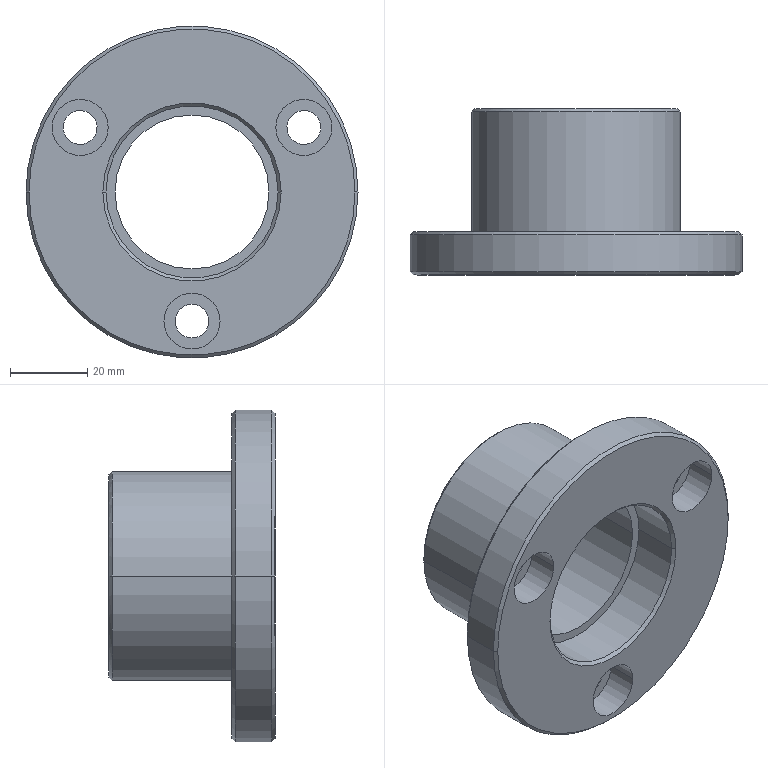Part | Creo | features CUT 4, CURVE 3, DATUM PLANE 3, CHAMFER 1, COORDINATE SYSTEM 1, PATTERN 1, PROTRUSION 1 | 1 solid | 40 faces | box 85.764 x 42.882 x 85.764 mm | volume 70979 mm3 | cylinder 22 | cone 10 | plane 8 | commonest cylinder face diameters 8.735 x6 14.5 x6 44.47 x4 39.777 x2 54 x2 85.764 x2
STEP:
#1=CARTESIAN_POINT('',(0.,0.,0.));
#2=DIRECTION('',(0.,0.,1.));
#3=DIRECTION('',(1.,0.,0.));
#4=AXIS2_PLACEMENT_3D('',#1,#2,#3);
#5=CARTESIAN_POINT('',(22.235,0.7941,0.));
#6=VERTEX_POINT('',#5);
#7=CARTESIAN_POINT('',(-22.235,0.7941,0.));
#8=VERTEX_POINT('',#7);
#9=CARTESIAN_POINT('',(0.,0.7941,0.));
#10=DIRECTION('',(0.,1.,0.));
#11=DIRECTION('',(1.,0.,0.));
#12=AXIS2_PLACEMENT_3D('',#9,#10,#11);
#13=CIRCLE('',#12,22.235);
#14=EDGE_CURVE('',#6,#8,#13,.T.);
#15=ORIENTED_EDGE('',*,*,#14,.T.);
#16=CARTESIAN_POINT('',(-22.235,12.706,0.));
#17=VERTEX_POINT('',#16);
#18=CARTESIAN_POINT('',(-22.235,12.706,0.));
#19=DIRECTION('',(0.,-1.,0.000000001));
#20=VECTOR('',#19,11.912);
#21=LINE('',#18,#20);
#22=EDGE_CURVE('',#17,#8,#21,.T.);
#23=ORIENTED_EDGE('',*,*,#22,.F.);
#24=CARTESIAN_POINT('',(22.235,12.706,0.));
#25=VERTEX_POINT('',#24);
#26=CARTESIAN_POINT('',(0.,12.706,0.));
#27=DIRECTION('',(0.,1.,0.));
#28=DIRECTION('',(1.,0.,0.));
#29=AXIS2_PLACEMENT_3D('',#26,#27,#28);
#30=CIRCLE('',#29,22.235);
#31=EDGE_CURVE('',#25,#17,#30,.T.);
#32=ORIENTED_EDGE('',*,*,#31,.F.);
#33=CARTESIAN_POINT('',(22.235,12.706,0.));
#34=DIRECTION('',(0.,-1.,-0.000000001));
#35=VECTOR('',#34,11.912);
#36=LINE('',#33,#35);
#37=EDGE_CURVE('',#25,#6,#36,.T.);
#38=ORIENTED_EDGE('',*,*,#37,.T.);
#39=EDGE_LOOP('',(#15,#23,#32,#38));
#40=FACE_OUTER_BOUND('',#39,.F.);
#41=CARTESIAN_POINT('',(0.,0.,0.));
#42=DIRECTION('',(0.,1.,0.));
#43=DIRECTION('',(1.,0.,0.));
#44=AXIS2_PLACEMENT_3D('',#41,#42,#43);
#45=CYLINDRICAL_SURFACE('',#44,22.235);
#46=ADVANCED_FACE('',(#40),#45,.F.);
#47=CARTESIAN_POINT('',(23.029,0.,0.));
#48=VERTEX_POINT('',#47);
#49=CARTESIAN_POINT('',(-23.029,0.,0.));
#50=VERTEX_POINT('',#49);
#51=CARTESIAN_POINT('',(0.,0.,0.));
#52=DIRECTION('',(0.,1.,0.));
#53=DIRECTION('',(1.,0.,0.));
#54=AXIS2_PLACEMENT_3D('',#51,#52,#53);
#55=CIRCLE('',#54,23.029);
#56=EDGE_CURVE('',#48,#50,#55,.T.);
#57=ORIENTED_EDGE('',*,*,#56,.T.);
#58=CARTESIAN_POINT('',(-23.029,0.000000001,0.000000013));
#59=DIRECTION('',(0.7071,0.7071,-0.000000003));
#60=VECTOR('',#59,1.123);
#61=LINE('',#58,#60);
#62=EDGE_CURVE('',#50,#8,#61,.T.);
#63=ORIENTED_EDGE('',*,*,#62,.T.);
#64=ORIENTED_EDGE('',*,*,#14,.F.);
#65=CARTESIAN_POINT('',(23.029,0.000000001,-0.000000013));
#66=DIRECTION('',(-0.7071,0.7071,0.000000003));
#67=VECTOR('',#66,1.123);
#68=LINE('',#65,#67);
#69=EDGE_CURVE('',#48,#6,#68,.T.);
#70=ORIENTED_EDGE('',*,*,#69,.F.);
#71=EDGE_LOOP('',(#57,#63,#64,#70));
#72=FACE_OUTER_BOUND('',#71,.F.);
#73=CARTESIAN_POINT('',(0.,0.3971,0.));
#74=DIRECTION('',(0.,-1.,0.));
#75=DIRECTION('',(0.,0.,-1.));
#76=AXIS2_PLACEMENT_3D('',#73,#74,#75);
#77=CONICAL_SURFACE('',#76,22.632,45.);
#78=ADVANCED_FACE('',(#72),#77,.F.);
#79=CARTESIAN_POINT('',(-42.088,0.,0.));
#80=VERTEX_POINT('',#79);
#81=CARTESIAN_POINT('',(42.088,0.,0.));
#82=VERTEX_POINT('',#81);
#83=CARTESIAN_POINT('',(0.,0.,0.));
#84=DIRECTION('',(0.,1.,0.));
#85=DIRECTION('',(-1.,0.,0.));
#86=AXIS2_PLACEMENT_3D('',#83,#84,#85);
#87=CIRCLE('',#86,42.088);
#88=EDGE_CURVE('',#80,#82,#87,.T.);
#89=ORIENTED_EDGE('',*,*,#88,.T.);
#90=CARTESIAN_POINT('',(0.,0.,0.));
#91=DIRECTION('',(0.,1.,0.));
#92=DIRECTION('',(1.,0.,0.));
#93=AXIS2_PLACEMENT_3D('',#90,#91,#92);
#94=CIRCLE('',#93,42.088);
#95=EDGE_CURVE('',#82,#80,#94,.T.);
#96=ORIENTED_EDGE('',*,*,#95,.T.);
#97=EDGE_LOOP('',(#89,#96));
#98=FACE_OUTER_BOUND('',#97,.F.);
#99=CARTESIAN_POINT('',(21.634,0.,16.676));
#100=VERTEX_POINT('',#99);
#101=CARTESIAN_POINT('',(36.134,0.,16.676));
#102=VERTEX_POINT('',#101);
#103=CARTESIAN_POINT('',(28.884,0.,16.676));
#104=DIRECTION('',(0.,-1.,0.));
#105=DIRECTION('',(-1.,0.,0.));
#106=AXIS2_PLACEMENT_3D('',#103,#104,#105);
#107=CIRCLE('',#106,7.25);
#108=EDGE_CURVE('',#100,#102,#107,.T.);
#109=ORIENTED_EDGE('',*,*,#108,.T.);
#110=CARTESIAN_POINT('',(28.884,0.,16.676));
#111=DIRECTION('',(0.,-1.,0.));
#112=DIRECTION('',(1.,0.,0.));
#113=AXIS2_PLACEMENT_3D('',#110,#111,#112);
#114=CIRCLE('',#113,7.25);
#115=EDGE_CURVE('',#102,#100,#114,.T.);
#116=ORIENTED_EDGE('',*,*,#115,.T.);
#117=EDGE_LOOP('',(#109,#116));
#118=FACE_BOUND('',#117,.F.);
#119=CARTESIAN_POINT('',(-36.134,0.,16.676));
#120=VERTEX_POINT('',#119);
#121=CARTESIAN_POINT('',(-21.634,0.,16.676));
#122=VERTEX_POINT('',#121);
#123=CARTESIAN_POINT('',(-28.884,0.,16.676));
#124=DIRECTION('',(0.,-1.,0.));
#125=DIRECTION('',(-1.,0.,0.));
#126=AXIS2_PLACEMENT_3D('',#123,#124,#125);
#127=CIRCLE('',#126,7.25);
#128=EDGE_CURVE('',#120,#122,#127,.T.);
#129=ORIENTED_EDGE('',*,*,#128,.T.);
#130=CARTESIAN_POINT('',(-28.884,0.,16.676));
#131=DIRECTION('',(0.,-1.,0.));
#132=DIRECTION('',(1.,0.,0.));
#133=AXIS2_PLACEMENT_3D('',#130,#131,#132);
#134=CIRCLE('',#133,7.25);
#135=EDGE_CURVE('',#122,#120,#134,.T.);
#136=ORIENTED_EDGE('',*,*,#135,.T.);
#137=EDGE_LOOP('',(#129,#136));
#138=FACE_BOUND('',#137,.F.);
#139=CARTESIAN_POINT('',(-7.25,0.,-33.353));
#140=VERTEX_POINT('',#139);
#141=CARTESIAN_POINT('',(7.25,0.,-33.353));
#142=VERTEX_POINT('',#141);
#143=CARTESIAN_POINT('',(0.,0.,-33.353));
#144=DIRECTION('',(0.,-1.,0.));
#145=DIRECTION('',(-1.,0.,0.));
#146=AXIS2_PLACEMENT_3D('',#143,#144,#145);
#147=CIRCLE('',#146,7.25);
#148=EDGE_CURVE('',#140,#142,#147,.T.);
#149=ORIENTED_EDGE('',*,*,#148,.T.);
#150=CARTESIAN_POINT('',(0.,0.,-33.353));
#151=DIRECTION('',(0.,-1.,0.));
#152=DIRECTION('',(1.,0.,0.));
#153=AXIS2_PLACEMENT_3D('',#150,#151,#152);
#154=CIRCLE('',#153,7.25);
#155=EDGE_CURVE('',#142,#140,#154,.T.);
#156=ORIENTED_EDGE('',*,*,#155,.T.);
#157=EDGE_LOOP('',(#149,#156));
#158=FACE_BOUND('',#157,.F.);
#159=CARTESIAN_POINT('',(0.,0.,0.));
#160=DIRECTION('',(0.,1.,0.));
#161=DIRECTION('',(-1.,0.,0.));
#162=AXIS2_PLACEMENT_3D('',#159,#160,#161);
#163=CIRCLE('',#162,23.029);
#164=EDGE_CURVE('',#50,#48,#163,.T.);
#165=ORIENTED_EDGE('',*,*,#164,.F.);
#166=ORIENTED_EDGE('',*,*,#56,.F.);
#167=EDGE_LOOP('',(#165,#166));
#168=FACE_BOUND('',#167,.F.);
#169=CARTESIAN_POINT('',(0.,0.,0.));
#170=DIRECTION('',(0.,1.,0.));
#171=DIRECTION('',(1.,0.,0.));
#172=AXIS2_PLACEMENT_3D('',#169,#170,#171);
#173=PLANE('',#172);
#174=ADVANCED_FACE('',(#98,#118,#138,#158,#168),#173,.F.);
#175=ORIENTED_EDGE('',*,*,#148,.F.);
#176=CARTESIAN_POINT('',(-7.25,7.941,-33.353));
#177=VERTEX_POINT('',#176);
#178=CARTESIAN_POINT('',(-7.25,0.,-33.353));
#179=DIRECTION('',(0.,1.,0.));
#180=VECTOR('',#179,7.941);
#181=LINE('',#178,#180);
#182=EDGE_CURVE('',#140,#177,#181,.T.);
#183=ORIENTED_EDGE('',*,*,#182,.T.);
#184=CARTESIAN_POINT('',(7.25,7.941,-33.353));
#185=VERTEX_POINT('',#184);
#186=CARTESIAN_POINT('',(0.,7.941,-33.353));
#187=DIRECTION('',(0.,-1.,0.));
#188=DIRECTION('',(-1.,0.,0.));
#189=AXIS2_PLACEMENT_3D('',#186,#187,#188);
#190=CIRCLE('',#189,7.25);
#191=EDGE_CURVE('',#177,#185,#190,.T.);
#192=ORIENTED_EDGE('',*,*,#191,.T.);
#193=CARTESIAN_POINT('',(7.25,0.,-33.353));
#194=DIRECTION('',(0.,1.,0.));
#195=VECTOR('',#194,7.941);
#196=LINE('',#193,#195);
#197=EDGE_CURVE('',#142,#185,#196,.T.);
#198=ORIENTED_EDGE('',*,*,#197,.F.);
#199=EDGE_LOOP('',(#175,#183,#192,#198));
#200=FACE_OUTER_BOUND('',#199,.F.);
#201=CARTESIAN_POINT('',(0.,0.,-33.353));
#202=DIRECTION('',(0.,-1.,0.));
#203=DIRECTION('',(-1.,0.,0.));
#204=AXIS2_PLACEMENT_3D('',#201,#202,#203);
#205=CYLINDRICAL_SURFACE('',#204,7.25);
#206=ADVANCED_FACE('',(#200),#205,.F.);
#207=ORIENTED_EDGE('',*,*,#155,.F.);
#208=ORIENTED_EDGE('',*,*,#197,.T.);
#209=CARTESIAN_POINT('',(0.,7.941,-33.353));
#210=DIRECTION('',(0.,-1.,0.));
#211=DIRECTION('',(1.,0.,0.));
#212=AXIS2_PLACEMENT_3D('',#209,#210,#211);
#213=CIRCLE('',#212,7.25);
#214=EDGE_CURVE('',#185,#177,#213,.T.);
#215=ORIENTED_EDGE('',*,*,#214,.T.);
#216=ORIENTED_EDGE('',*,*,#182,.F.);
#217=EDGE_LOOP('',(#207,#208,#215,#216));
#218=FACE_OUTER_BOUND('',#217,.F.);
#219=CARTESIAN_POINT('',(0.,0.,-33.353));
#220=DIRECTION('',(0.,-1.,0.));
#221=DIRECTION('',(-1.,0.,0.));
#222=AXIS2_PLACEMENT_3D('',#219,#220,#221);
#223=CYLINDRICAL_SURFACE('',#222,7.25);
#224=ADVANCED_FACE('',(#218),#223,.F.);
#225=ORIENTED_EDGE('',*,*,#191,.F.);
#226=ORIENTED_EDGE('',*,*,#214,.F.);
#227=EDGE_LOOP('',(#225,#226));
#228=FACE_OUTER_BOUND('',#227,.F.);
#229=CARTESIAN_POINT('',(4.368,7.941,-33.353));
#230=VERTEX_POINT('',#229);
#231=CARTESIAN_POINT('',(-4.368,7.941,-33.353));
#232=VERTEX_POINT('',#231);
#233=CARTESIAN_POINT('',(0.,7.941,-33.353));
#234=DIRECTION('',(0.,1.,0.));
#235=DIRECTION('',(1.,0.,0.));
#236=AXIS2_PLACEMENT_3D('',#233,#234,#235);
#237=CIRCLE('',#236,4.368);
#238=EDGE_CURVE('',#230,#232,#237,.T.);
#239=ORIENTED_EDGE('',*,*,#238,.F.);
#240=CARTESIAN_POINT('',(0.,7.941,-33.353));
#241=DIRECTION('',(0.,1.,0.));
#242=DIRECTION('',(-1.,0.,0.));
#243=AXIS2_PLACEMENT_3D('',#240,#241,#242);
#244=CIRCLE('',#243,4.368);
#245=EDGE_CURVE('',#232,#230,#244,.T.);
#246=ORIENTED_EDGE('',*,*,#245,.F.);
#247=EDGE_LOOP('',(#239,#246));
#248=FACE_BOUND('',#247,.F.);
#249=CARTESIAN_POINT('',(0.,7.941,0.));
#250=DIRECTION('',(0.,-1.,0.));
#251=DIRECTION('',(-1.,0.,0.));
#252=AXIS2_PLACEMENT_3D('',#249,#250,#251);
#253=PLANE('',#252);
#254=ADVANCED_FACE('',(#228,#248),#253,.T.);
#255=CARTESIAN_POINT('',(21.634,7.941,16.676));
#256=VERTEX_POINT('',#255);
#257=CARTESIAN_POINT('',(36.134,7.941,16.676));
#258=VERTEX_POINT('',#257);
#259=CARTESIAN_POINT('',(28.884,7.941,16.676));
#260=DIRECTION('',(0.,-1.,0.));
#261=DIRECTION('',(-1.,0.,0.));
#262=AXIS2_PLACEMENT_3D('',#259,#260,#261);
#263=CIRCLE('',#262,7.25);
#264=EDGE_CURVE('',#256,#258,#263,.T.);
#265=ORIENTED_EDGE('',*,*,#264,.F.);
#266=CARTESIAN_POINT('',(28.884,7.941,16.676));
#267=DIRECTION('',(0.,-1.,0.));
#268=DIRECTION('',(1.,0.,0.));
#269=AXIS2_PLACEMENT_3D('',#266,#267,#268);
#270=CIRCLE('',#269,7.25);
#271=EDGE_CURVE('',#258,#256,#270,.T.);
#272=ORIENTED_EDGE('',*,*,#271,.F.);
#273=EDGE_LOOP('',(#265,#272));
#274=FACE_OUTER_BOUND('',#273,.F.);
#275=CARTESIAN_POINT('',(26.701,7.941,20.459));
#276=VERTEX_POINT('',#275);
#277=CARTESIAN_POINT('',(31.068,7.941,12.894));
#278=VERTEX_POINT('',#277);
#279=CARTESIAN_POINT('',(28.884,7.941,16.676));
#280=DIRECTION('',(0.,1.,0.));
#281=DIRECTION('',(-0.5,0.,0.866));
#282=AXIS2_PLACEMENT_3D('',#279,#280,#281);
#283=CIRCLE('',#282,4.368);
#284=EDGE_CURVE('',#276,#278,#283,.T.);
#285=ORIENTED_EDGE('',*,*,#284,.F.);
#286=CARTESIAN_POINT('',(28.884,7.941,16.676));
#287=DIRECTION('',(0.,1.,0.));
#288=DIRECTION('',(0.5,0.,-0.866));
#289=AXIS2_PLACEMENT_3D('',#286,#287,#288);
#290=CIRCLE('',#289,4.368);
#291=EDGE_CURVE('',#278,#276,#290,.T.);
#292=ORIENTED_EDGE('',*,*,#291,.F.);
#293=EDGE_LOOP('',(#285,#292));
#294=FACE_BOUND('',#293,.F.);
#295=CARTESIAN_POINT('',(0.,7.941,0.));
#296=DIRECTION('',(0.,-1.,0.));
#297=DIRECTION('',(-1.,0.,0.));
#298=AXIS2_PLACEMENT_3D('',#295,#296,#297);
#299=PLANE('',#298);
#300=ADVANCED_FACE('',(#274,#294),#299,.T.);
#301=CARTESIAN_POINT('',(-36.134,7.941,16.676));
#302=VERTEX_POINT('',#301);
#303=CARTESIAN_POINT('',(-21.634,7.941,16.676));
#304=VERTEX_POINT('',#303);
#305=CARTESIAN_POINT('',(-28.884,7.941,16.676));
#306=DIRECTION('',(0.,-1.,0.));
#307=DIRECTION('',(-1.,0.,0.));
#308=AXIS2_PLACEMENT_3D('',#305,#306,#307);
#309=CIRCLE('',#308,7.25);
#310=EDGE_CURVE('',#302,#304,#309,.T.);
#311=ORIENTED_EDGE('',*,*,#310,.F.);
#312=CARTESIAN_POINT('',(-28.884,7.941,16.676));
#313=DIRECTION('',(0.,-1.,0.));
#314=DIRECTION('',(1.,0.,0.));
#315=AXIS2_PLACEMENT_3D('',#312,#313,#314);
#316=CIRCLE('',#315,7.25);
#317=EDGE_CURVE('',#304,#302,#316,.T.);
#318=ORIENTED_EDGE('',*,*,#317,.F.);
#319=EDGE_LOOP('',(#311,#318));
#320=FACE_OUTER_BOUND('',#319,.F.);
#321=CARTESIAN_POINT('',(-31.068,7.941,12.894));
#322=VERTEX_POINT('',#321);
#323=CARTESIAN_POINT('',(-26.701,7.941,20.459));
#324=VERTEX_POINT('',#323);
#325=CARTESIAN_POINT('',(-28.884,7.941,16.676));
#326=DIRECTION('',(0.,1.,0.));
#327=DIRECTION('',(-0.5,0.,-0.866));
#328=AXIS2_PLACEMENT_3D('',#325,#326,#327);
#329=CIRCLE('',#328,4.368);
#330=EDGE_CURVE('',#322,#324,#329,.T.);
#331=ORIENTED_EDGE('',*,*,#330,.F.);
#332=CARTESIAN_POINT('',(-28.884,7.941,16.676));
#333=DIRECTION('',(0.,1.,0.));
#334=DIRECTION('',(0.5,0.,0.866));
#335=AXIS2_PLACEMENT_3D('',#332,#333,#334);
#336=CIRCLE('',#335,4.368);
#337=EDGE_CURVE('',#324,#322,#336,.T.);
#338=ORIENTED_EDGE('',*,*,#337,.F.);
#339=EDGE_LOOP('',(#331,#338));
#340=FACE_BOUND('',#339,.F.);
#341=CARTESIAN_POINT('',(0.,7.941,0.));
#342=DIRECTION('',(0.,-1.,0.));
#343=DIRECTION('',(-1.,0.,0.));
#344=AXIS2_PLACEMENT_3D('',#341,#342,#343);
#345=PLANE('',#344);
#346=ADVANCED_FACE('',(#320,#340),#345,.T.);
#347=ORIENTED_EDGE('',*,*,#108,.F.);
#348=CARTESIAN_POINT('',(21.634,0.,16.676));
#349=DIRECTION('',(0.,1.,0.));
#350=VECTOR('',#349,7.941);
#351=LINE('',#348,#350);
#352=EDGE_CURVE('',#100,#256,#351,.T.);
#353=ORIENTED_EDGE('',*,*,#352,.T.);
#354=ORIENTED_EDGE('',*,*,#264,.T.);
#355=CARTESIAN_POINT('',(36.134,0.,16.676));
#356=DIRECTION('',(0.,1.,0.));
#357=VECTOR('',#356,7.941);
#358=LINE('',#355,#357);
#359=EDGE_CURVE('',#102,#258,#358,.T.);
#360=ORIENTED_EDGE('',*,*,#359,.F.);
#361=EDGE_LOOP('',(#347,#353,#354,#360));
#362=FACE_OUTER_BOUND('',#361,.F.);
#363=CARTESIAN_POINT('',(28.884,0.,16.676));
#364=DIRECTION('',(0.,-1.,0.));
#365=DIRECTION('',(-1.,0.,0.));
#366=AXIS2_PLACEMENT_3D('',#363,#364,#365);
#367=CYLINDRICAL_SURFACE('',#366,7.25);
#368=ADVANCED_FACE('',(#362),#367,.F.);
#369=ORIENTED_EDGE('',*,*,#115,.F.);
#370=ORIENTED_EDGE('',*,*,#359,.T.);
#371=ORIENTED_EDGE('',*,*,#271,.T.);
#372=ORIENTED_EDGE('',*,*,#352,.F.);
#373=EDGE_LOOP('',(#369,#370,#371,#372));
#374=FACE_OUTER_BOUND('',#373,.F.);
#375=CARTESIAN_POINT('',(28.884,0.,16.676));
#376=DIRECTION('',(0.,-1.,0.));
#377=DIRECTION('',(-1.,0.,0.));
#378=AXIS2_PLACEMENT_3D('',#375,#376,#377);
#379=CYLINDRICAL_SURFACE('',#378,7.25);
#380=ADVANCED_FACE('',(#374),#379,.F.);
#381=ORIENTED_EDGE('',*,*,#128,.F.);
#382=CARTESIAN_POINT('',(-36.134,0.,16.676));
#383=DIRECTION('',(0.,1.,0.));
#384=VECTOR('',#383,7.941);
#385=LINE('',#382,#384);
#386=EDGE_CURVE('',#120,#302,#385,.T.);
#387=ORIENTED_EDGE('',*,*,#386,.T.);
#388=ORIENTED_EDGE('',*,*,#310,.T.);
#389=CARTESIAN_POINT('',(-21.634,0.,16.676));
#390=DIRECTION('',(0.,1.,0.));
#391=VECTOR('',#390,7.941);
#392=LINE('',#389,#391);
#393=EDGE_CURVE('',#122,#304,#392,.T.);
#394=ORIENTED_EDGE('',*,*,#393,.F.);
#395=EDGE_LOOP('',(#381,#387,#388,#394));
#396=FACE_OUTER_BOUND('',#395,.F.);
#397=CARTESIAN_POINT('',(-28.884,0.,16.676));
#398=DIRECTION('',(0.,-1.,0.));
#399=DIRECTION('',(-1.,0.,0.));
#400=AXIS2_PLACEMENT_3D('',#397,#398,#399);
#401=CYLINDRICAL_SURFACE('',#400,7.25);
#402=ADVANCED_FACE('',(#396),#401,.F.);
#403=ORIENTED_EDGE('',*,*,#135,.F.);
#404=ORIENTED_EDGE('',*,*,#393,.T.);
#405=ORIENTED_EDGE('',*,*,#317,.T.);
#406=ORIENTED_EDGE('',*,*,#386,.F.);
#407=EDGE_LOOP('',(#403,#404,#405,#406));
#408=FACE_OUTER_BOUND('',#407,.F.);
#409=CARTESIAN_POINT('',(-28.884,0.,16.676));
#410=DIRECTION('',(0.,-1.,0.));
#411=DIRECTION('',(-1.,0.,0.));
#412=AXIS2_PLACEMENT_3D('',#409,#410,#411);
#413=CYLINDRICAL_SURFACE('',#412,7.25);
#414=ADVANCED_FACE('',(#408),#413,.F.);
#415=ORIENTED_EDGE('',*,*,#238,.T.);
#416=CARTESIAN_POINT('',(-4.368,11.118,-33.353));
#417=VERTEX_POINT('',#416);
#418=CARTESIAN_POINT('',(-4.368,11.118,-33.353));
#419=DIRECTION('',(0.,-1.,0.));
#420=VECTOR('',#419,3.176);
#421=LINE('',#418,#420);
#422=EDGE_CURVE('',#417,#232,#421,.T.);
#423=ORIENTED_EDGE('',*,*,#422,.F.);
#424=CARTESIAN_POINT('',(4.368,11.118,-33.353));
#425=VERTEX_POINT('',#424);
#426=CARTESIAN_POINT('',(0.,11.118,-33.353));
#427=DIRECTION('',(0.,1.,0.));
#428=DIRECTION('',(1.,0.,0.));
#429=AXIS2_PLACEMENT_3D('',#426,#427,#428);
#430=CIRCLE('',#429,4.368);
#431=EDGE_CURVE('',#425,#417,#430,.T.);
#432=ORIENTED_EDGE('',*,*,#431,.F.);
#433=CARTESIAN_POINT('',(4.368,11.118,-33.353));
#434=DIRECTION('',(0.,-1.,0.));
#435=VECTOR('',#434,3.176);
#436=LINE('',#433,#435);
#437=EDGE_CURVE('',#425,#230,#436,.T.);
#438=ORIENTED_EDGE('',*,*,#437,.T.);
#439=EDGE_LOOP('',(#415,#423,#432,#438));
#440=FACE_OUTER_BOUND('',#439,.F.);
#441=CARTESIAN_POINT('',(0.,11.118,-33.353));
#442=DIRECTION('',(0.,1.,0.));
#443=DIRECTION('',(1.,0.,0.));
#444=AXIS2_PLACEMENT_3D('',#441,#442,#443);
#445=CYLINDRICAL_SURFACE('',#444,4.368);
#446=ADVANCED_FACE('',(#440),#445,.F.);
#447=ORIENTED_EDGE('',*,*,#245,.T.);
#448=ORIENTED_EDGE('',*,*,#437,.F.);
#449=CARTESIAN_POINT('',(0.,11.118,-33.353));
#450=DIRECTION('',(0.,1.,0.));
#451=DIRECTION('',(-1.,0.,0.));
#452=AXIS2_PLACEMENT_3D('',#449,#450,#451);
#453=CIRCLE('',#452,4.368);
#454=EDGE_CURVE('',#417,#425,#453,.T.);
#455=ORIENTED_EDGE('',*,*,#454,.F.);
#456=ORIENTED_EDGE('',*,*,#422,.T.);
#457=EDGE_LOOP('',(#447,#448,#455,#456));
#458=FACE_OUTER_BOUND('',#457,.F.);
#459=CARTESIAN_POINT('',(0.,11.118,-33.353));
#460=DIRECTION('',(0.,1.,0.));
#461=DIRECTION('',(1.,0.,0.));
#462=AXIS2_PLACEMENT_3D('',#459,#460,#461);
#463=CYLINDRICAL_SURFACE('',#462,4.368);
#464=ADVANCED_FACE('',(#458),#463,.F.);
#465=CARTESIAN_POINT('',(-42.088,11.118,0.));
#466=VERTEX_POINT('',#465);
#467=CARTESIAN_POINT('',(42.088,11.118,0.));
#468=VERTEX_POINT('',#467);
#469=CARTESIAN_POINT('',(0.,11.118,0.));
#470=DIRECTION('',(0.,1.,0.));
#471=DIRECTION('',(-1.,0.,0.));
#472=AXIS2_PLACEMENT_3D('',#469,#470,#471);
#473=CIRCLE('',#472,42.088);
#474=EDGE_CURVE('',#466,#468,#473,.T.);
#475=ORIENTED_EDGE('',*,*,#474,.F.);
#476=CARTESIAN_POINT('',(0.,11.118,0.));
#477=DIRECTION('',(0.,1.,0.));
#478=DIRECTION('',(1.,0.,0.));
#479=AXIS2_PLACEMENT_3D('',#476,#477,#478);
#480=CIRCLE('',#479,42.088);
#481=EDGE_CURVE('',#468,#466,#480,.T.);
#482=ORIENTED_EDGE('',*,*,#481,.F.);
#483=EDGE_LOOP('',(#475,#482));
#484=FACE_OUTER_BOUND('',#483,.F.);
#485=ORIENTED_EDGE('',*,*,#431,.T.);
#486=ORIENTED_EDGE('',*,*,#454,.T.);
#487=EDGE_LOOP('',(#485,#486));
#488=FACE_BOUND('',#487,.F.);
#489=CARTESIAN_POINT('',(-31.068,11.118,12.894));
#490=VERTEX_POINT('',#489);
#491=CARTESIAN_POINT('',(-26.701,11.118,20.459));
#492=VERTEX_POINT('',#491);
#493=CARTESIAN_POINT('',(-28.884,11.118,16.676));
#494=DIRECTION('',(0.,1.,0.));
#495=DIRECTION('',(-0.5,0.,-0.866));
#496=AXIS2_PLACEMENT_3D('',#493,#494,#495);
#497=CIRCLE('',#496,4.368);
#498=EDGE_CURVE('',#490,#492,#497,.T.);
#499=ORIENTED_EDGE('',*,*,#498,.T.);
#500=CARTESIAN_POINT('',(-28.884,11.118,16.676));
#501=DIRECTION('',(0.,1.,0.));
#502=DIRECTION('',(0.5,0.,0.866));
#503=AXIS2_PLACEMENT_3D('',#500,#501,#502);
#504=CIRCLE('',#503,4.368);
#505=EDGE_CURVE('',#492,#490,#504,.T.);
#506=ORIENTED_EDGE('',*,*,#505,.T.);
#507=EDGE_LOOP('',(#499,#506));
#508=FACE_BOUND('',#507,.F.);
#509=CARTESIAN_POINT('',(26.701,11.118,20.459));
#510=VERTEX_POINT('',#509);
#511=CARTESIAN_POINT('',(31.068,11.118,12.894));
#512=VERTEX_POINT('',#511);
#513=CARTESIAN_POINT('',(28.884,11.118,16.676));
#514=DIRECTION('',(0.,1.,0.));
#515=DIRECTION('',(-0.5,0.,0.866));
#516=AXIS2_PLACEMENT_3D('',#513,#514,#515);
#517=CIRCLE('',#516,4.368);
#518=EDGE_CURVE('',#510,#512,#517,.T.);
#519=ORIENTED_EDGE('',*,*,#518,.T.);
#520=CARTESIAN_POINT('',(28.884,11.118,16.676));
#521=DIRECTION('',(0.,1.,0.));
#522=DIRECTION('',(0.5,0.,-0.866));
#523=AXIS2_PLACEMENT_3D('',#520,#521,#522);
#524=CIRCLE('',#523,4.368);
#525=EDGE_CURVE('',#512,#510,#524,.T.);
#526=ORIENTED_EDGE('',*,*,#525,.T.);
#527=EDGE_LOOP('',(#519,#526));
#528=FACE_BOUND('',#527,.F.);
#529=CARTESIAN_POINT('',(27.,11.118,0.));
#530=VERTEX_POINT('',#529);
#531=CARTESIAN_POINT('',(-27.,11.118,0.));
#532=VERTEX_POINT('',#531);
#533=CARTESIAN_POINT('',(0.,11.118,0.));
#534=DIRECTION('',(0.,-1.,0.));
#535=DIRECTION('',(1.,0.,0.));
#536=AXIS2_PLACEMENT_3D('',#533,#534,#535);
#537=CIRCLE('',#536,27.);
#538=EDGE_CURVE('',#530,#532,#537,.T.);
#539=ORIENTED_EDGE('',*,*,#538,.F.);
#540=CARTESIAN_POINT('',(0.,11.118,0.));
#541=DIRECTION('',(0.,1.,0.));
#542=DIRECTION('',(1.,0.,0.));
#543=AXIS2_PLACEMENT_3D('',#540,#541,#542);
#544=CIRCLE('',#543,27.);
#545=EDGE_CURVE('',#530,#532,#544,.T.);
#546=ORIENTED_EDGE('',*,*,#545,.T.);
#547=EDGE_LOOP('',(#539,#546));
#548=FACE_BOUND('',#547,.F.);
#549=CARTESIAN_POINT('',(0.,11.118,0.));
#550=DIRECTION('',(0.,1.,0.));
#551=DIRECTION('',(1.,0.,0.));
#552=AXIS2_PLACEMENT_3D('',#549,#550,#551);
#553=PLANE('',#552);
#554=ADVANCED_FACE('',(#484,#488,#508,#528,#548),#553,.T.);
#555=CARTESIAN_POINT('',(-27.,42.088,0.));
#556=VERTEX_POINT('',#555);
#557=CARTESIAN_POINT('',(27.,42.088,0.));
#558=VERTEX_POINT('',#557);
#559=CARTESIAN_POINT('',(0.,42.088,0.));
#560=DIRECTION('',(0.,1.,0.));
#561=DIRECTION('',(-1.,0.,0.));
#562=AXIS2_PLACEMENT_3D('',#559,#560,#561);
#563=CIRCLE('',#562,27.);
#564=EDGE_CURVE('',#556,#558,#563,.T.);
#565=ORIENTED_EDGE('',*,*,#564,.T.);
#566=CARTESIAN_POINT('',(27.,11.118,0.));
#567=DIRECTION('',(0.,1.,0.));
#568=VECTOR('',#567,30.97);
#569=LINE('',#566,#568);
#570=EDGE_CURVE('',#530,#558,#569,.T.);
#571=ORIENTED_EDGE('',*,*,#570,.F.);
#572=ORIENTED_EDGE('',*,*,#538,.T.);
#573=CARTESIAN_POINT('',(-27.,11.118,0.));
#574=DIRECTION('',(0.,1.,0.));
#575=VECTOR('',#574,30.97);
#576=LINE('',#573,#575);
#577=EDGE_CURVE('',#532,#556,#576,.T.);
#578=ORIENTED_EDGE('',*,*,#577,.T.);
#579=EDGE_LOOP('',(#565,#571,#572,#578));
#580=FACE_OUTER_BOUND('',#579,.F.);
#581=CARTESIAN_POINT('',(0.,0.,0.));
#582=DIRECTION('',(0.,1.,0.));
#583=DIRECTION('',(1.,0.,0.));
#584=AXIS2_PLACEMENT_3D('',#581,#582,#583);
#585=CYLINDRICAL_SURFACE('',#584,27.);
#586=ADVANCED_FACE('',(#580),#585,.T.);
#587=CARTESIAN_POINT('',(-26.206,42.882,0.));
#588=VERTEX_POINT('',#587);
#589=CARTESIAN_POINT('',(26.206,42.882,0.));
#590=VERTEX_POINT('',#589);
#591=CARTESIAN_POINT('',(0.,42.882,0.));
#592=DIRECTION('',(0.,1.,0.));
#593=DIRECTION('',(-1.,0.,0.));
#594=AXIS2_PLACEMENT_3D('',#591,#592,#593);
#595=CIRCLE('',#594,26.206);
#596=EDGE_CURVE('',#588,#590,#595,.T.);
#597=ORIENTED_EDGE('',*,*,#596,.T.);
#598=CARTESIAN_POINT('',(26.206,42.882,-0.000000007));
#599=DIRECTION('',(0.7071,-0.7071,0.000000001));
#600=VECTOR('',#599,1.123);
#601=LINE('',#598,#600);
#602=EDGE_CURVE('',#590,#558,#601,.T.);
#603=ORIENTED_EDGE('',*,*,#602,.T.);
#604=ORIENTED_EDGE('',*,*,#564,.F.);
#605=CARTESIAN_POINT('',(-26.206,42.882,0.000000007));
#606=DIRECTION('',(-0.7071,-0.7071,-0.000000001));
#607=VECTOR('',#606,1.123);
#608=LINE('',#605,#607);
#609=EDGE_CURVE('',#588,#556,#608,.T.);
#610=ORIENTED_EDGE('',*,*,#609,.F.);
#611=EDGE_LOOP('',(#597,#603,#604,#610));
#612=FACE_OUTER_BOUND('',#611,.F.);
#613=CARTESIAN_POINT('',(0.,42.485,0.));
#614=DIRECTION('',(0.,-1.,0.));
#615=DIRECTION('',(0.,0.,-1.));
#616=AXIS2_PLACEMENT_3D('',#613,#614,#615);
#617=CONICAL_SURFACE('',#616,26.603,45.);
#618=ADVANCED_FACE('',(#612),#617,.T.);
#619=ORIENTED_EDGE('',*,*,#596,.F.);
#620=CARTESIAN_POINT('',(0.,42.882,0.));
#621=DIRECTION('',(0.,1.,0.));
#622=DIRECTION('',(1.,0.,0.));
#623=AXIS2_PLACEMENT_3D('',#620,#621,#622);
#624=CIRCLE('',#623,26.206);
#625=EDGE_CURVE('',#590,#588,#624,.T.);
#626=ORIENTED_EDGE('',*,*,#625,.F.);
#627=EDGE_LOOP('',(#619,#626));
#628=FACE_OUTER_BOUND('',#627,.F.);
#629=CARTESIAN_POINT('',(-23.029,42.882,0.));
#630=VERTEX_POINT('',#629);
#631=CARTESIAN_POINT('',(23.029,42.882,0.));
#632=VERTEX_POINT('',#631);
#633=CARTESIAN_POINT('',(0.,42.882,0.));
#634=DIRECTION('',(0.,1.,0.));
#635=DIRECTION('',(-1.,0.,0.));
#636=AXIS2_PLACEMENT_3D('',#633,#634,#635);
#637=CIRCLE('',#636,23.029);
#638=EDGE_CURVE('',#630,#632,#637,.T.);
#639=ORIENTED_EDGE('',*,*,#638,.T.);
#640=CARTESIAN_POINT('',(0.,42.882,0.));
#641=DIRECTION('',(0.,1.,0.));
#642=DIRECTION('',(1.,0.,0.));
#643=AXIS2_PLACEMENT_3D('',#640,#641,#642);
#644=CIRCLE('',#643,23.029);
#645=EDGE_CURVE('',#632,#630,#644,.T.);
#646=ORIENTED_EDGE('',*,*,#645,.T.);
#647=EDGE_LOOP('',(#639,#646));
#648=FACE_BOUND('',#647,.F.);
#649=CARTESIAN_POINT('',(0.,42.882,0.));
#650=DIRECTION('',(0.,1.,0.));
#651=DIRECTION('',(1.,0.,0.));
#652=AXIS2_PLACEMENT_3D('',#649,#650,#651);
#653=PLANE('',#652);
#654=ADVANCED_FACE('',(#628,#648),#653,.T.);
#655=ORIENTED_EDGE('',*,*,#625,.T.);
#656=ORIENTED_EDGE('',*,*,#609,.T.);
#657=CARTESIAN_POINT('',(0.,42.088,0.));
#658=DIRECTION('',(0.,1.,0.));
#659=DIRECTION('',(1.,0.,0.));
#660=AXIS2_PLACEMENT_3D('',#657,#658,#659);
#661=CIRCLE('',#660,27.);
#662=EDGE_CURVE('',#558,#556,#661,.T.);
#663=ORIENTED_EDGE('',*,*,#662,.F.);
#664=ORIENTED_EDGE('',*,*,#602,.F.);
#665=EDGE_LOOP('',(#655,#656,#663,#664));
#666=FACE_OUTER_BOUND('',#665,.F.);
#667=CARTESIAN_POINT('',(0.,42.485,0.));
#668=DIRECTION('',(0.,-1.,0.));
#669=DIRECTION('',(0.,0.,-1.));
#670=AXIS2_PLACEMENT_3D('',#667,#668,#669);
#671=CONICAL_SURFACE('',#670,26.603,45.);
#672=ADVANCED_FACE('',(#666),#671,.T.);
#673=ORIENTED_EDGE('',*,*,#662,.T.);
#674=ORIENTED_EDGE('',*,*,#577,.F.);
#675=ORIENTED_EDGE('',*,*,#545,.F.);
#676=ORIENTED_EDGE('',*,*,#570,.T.);
#677=EDGE_LOOP('',(#673,#674,#675,#676));
#678=FACE_OUTER_BOUND('',#677,.F.);
#679=CARTESIAN_POINT('',(0.,0.,0.));
#680=DIRECTION('',(0.,1.,0.));
#681=DIRECTION('',(1.,0.,0.));
#682=AXIS2_PLACEMENT_3D('',#679,#680,#681);
#683=CYLINDRICAL_SURFACE('',#682,27.);
#684=ADVANCED_FACE('',(#678),#683,.T.);
#685=CARTESIAN_POINT('',(-22.235,42.088,0.));
#686=VERTEX_POINT('',#685);
#687=CARTESIAN_POINT('',(22.235,42.088,0.));
#688=VERTEX_POINT('',#687);
#689=CARTESIAN_POINT('',(0.,42.088,0.));
#690=DIRECTION('',(0.,1.,0.));
#691=DIRECTION('',(-1.,0.,0.));
#692=AXIS2_PLACEMENT_3D('',#689,#690,#691);
#693=CIRCLE('',#692,22.235);
#694=EDGE_CURVE('',#686,#688,#693,.T.);
#695=ORIENTED_EDGE('',*,*,#694,.T.);
#696=CARTESIAN_POINT('',(22.235,42.088,0.000000002));
#697=DIRECTION('',(0.7071,0.7071,0.000000001));
#698=VECTOR('',#697,1.123);
#699=LINE('',#696,#698);
#700=EDGE_CURVE('',#688,#632,#699,.T.);
#701=ORIENTED_EDGE('',*,*,#700,.T.);
#702=ORIENTED_EDGE('',*,*,#638,.F.);
#703=CARTESIAN_POINT('',(-22.235,42.088,-0.000000002));
#704=DIRECTION('',(-0.7071,0.7071,-0.000000001));
#705=VECTOR('',#704,1.123);
#706=LINE('',#703,#705);
#707=EDGE_CURVE('',#686,#630,#706,.T.);
#708=ORIENTED_EDGE('',*,*,#707,.F.);
#709=EDGE_LOOP('',(#695,#701,#702,#708));
#710=FACE_OUTER_BOUND('',#709,.F.);
#711=CARTESIAN_POINT('',(0.,42.485,0.));
#712=DIRECTION('',(0.,1.,0.));
#713=DIRECTION('',(0.,0.,-1.));
#714=AXIS2_PLACEMENT_3D('',#711,#712,#713);
#715=CONICAL_SURFACE('',#714,22.632,45.);
#716=ADVANCED_FACE('',(#710),#715,.F.);
#717=ORIENTED_EDGE('',*,*,#694,.F.);
#718=CARTESIAN_POINT('',(-22.235,30.176,0.));
#719=VERTEX_POINT('',#718);
#720=CARTESIAN_POINT('',(-22.235,42.088,-0.000000002));
#721=DIRECTION('',(0.,-1.,0.));
#722=VECTOR('',#721,11.912);
#723=LINE('',#720,#722);
#724=EDGE_CURVE('',#686,#719,#723,.T.);
#725=ORIENTED_EDGE('',*,*,#724,.T.);
#726=CARTESIAN_POINT('',(22.235,30.176,0.));
#727=VERTEX_POINT('',#726);
#728=CARTESIAN_POINT('',(0.,30.176,0.));
#729=DIRECTION('',(0.,-1.,0.));
#730=DIRECTION('',(1.,0.,0.));
#731=AXIS2_PLACEMENT_3D('',#728,#729,#730);
#732=CIRCLE('',#731,22.235);
#733=EDGE_CURVE('',#727,#719,#732,.T.);
#734=ORIENTED_EDGE('',*,*,#733,.F.);
#735=CARTESIAN_POINT('',(22.235,42.088,0.000000002));
#736=DIRECTION('',(0.,-1.,0.));
#737=VECTOR('',#736,11.912);
#738=LINE('',#735,#737);
#739=EDGE_CURVE('',#688,#727,#738,.T.);
#740=ORIENTED_EDGE('',*,*,#739,.F.);
#741=EDGE_LOOP('',(#717,#725,#734,#740));
#742=FACE_OUTER_BOUND('',#741,.F.);
#743=CARTESIAN_POINT('',(0.,0.,0.));
#744=DIRECTION('',(0.,1.,0.));
#745=DIRECTION('',(1.,0.,0.));
#746=AXIS2_PLACEMENT_3D('',#743,#744,#745);
#747=CYLINDRICAL_SURFACE('',#746,22.235);
#748=ADVANCED_FACE('',(#742),#747,.F.);
#749=CARTESIAN_POINT('',(0.,42.088,0.));
#750=DIRECTION('',(0.,1.,0.));
#751=DIRECTION('',(1.,0.,0.));
#752=AXIS2_PLACEMENT_3D('',#749,#750,#751);
#753=CIRCLE('',#752,22.235);
#754=EDGE_CURVE('',#688,#686,#753,.T.);
#755=ORIENTED_EDGE('',*,*,#754,.F.);
#756=ORIENTED_EDGE('',*,*,#739,.T.);
#757=CARTESIAN_POINT('',(0.,30.176,0.));
#758=DIRECTION('',(0.,1.,0.));
#759=DIRECTION('',(1.,0.,0.));
#760=AXIS2_PLACEMENT_3D('',#757,#758,#759);
#761=CIRCLE('',#760,22.235);
#762=EDGE_CURVE('',#727,#719,#761,.T.);
#763=ORIENTED_EDGE('',*,*,#762,.T.);
#764=ORIENTED_EDGE('',*,*,#724,.F.);
#765=EDGE_LOOP('',(#755,#756,#763,#764));
#766=FACE_OUTER_BOUND('',#765,.F.);
#767=CARTESIAN_POINT('',(0.,0.,0.));
#768=DIRECTION('',(0.,1.,0.));
#769=DIRECTION('',(1.,0.,0.));
#770=AXIS2_PLACEMENT_3D('',#767,#768,#769);
#771=CYLINDRICAL_SURFACE('',#770,22.235);
#772=ADVANCED_FACE('',(#766),#771,.F.);
#773=ORIENTED_EDGE('',*,*,#754,.T.);
#774=ORIENTED_EDGE('',*,*,#707,.T.);
#775=ORIENTED_EDGE('',*,*,#645,.F.);
#776=ORIENTED_EDGE('',*,*,#700,.F.);
#777=EDGE_LOOP('',(#773,#774,#775,#776));
#778=FACE_OUTER_BOUND('',#777,.F.);
#779=CARTESIAN_POINT('',(0.,42.485,0.));
#780=DIRECTION('',(0.,1.,0.));
#781=DIRECTION('',(0.,0.,-1.));
#782=AXIS2_PLACEMENT_3D('',#779,#780,#781);
#783=CONICAL_SURFACE('',#782,22.632,45.);
#784=ADVANCED_FACE('',(#778),#783,.F.);
#785=ORIENTED_EDGE('',*,*,#762,.F.);
#786=ORIENTED_EDGE('',*,*,#733,.T.);
#787=EDGE_LOOP('',(#785,#786));
#788=FACE_OUTER_BOUND('',#787,.F.);
#789=CARTESIAN_POINT('',(19.888,30.176,0.));
#790=VERTEX_POINT('',#789);
#791=CARTESIAN_POINT('',(-19.888,30.176,0.));
#792=VERTEX_POINT('',#791);
#793=CARTESIAN_POINT('',(0.,30.176,0.));
#794=DIRECTION('',(0.,-1.,0.));
#795=DIRECTION('',(1.,0.,0.));
#796=AXIS2_PLACEMENT_3D('',#793,#794,#795);
#797=CIRCLE('',#796,19.888);
#798=EDGE_CURVE('',#790,#792,#797,.T.);
#799=ORIENTED_EDGE('',*,*,#798,.F.);
#800=CARTESIAN_POINT('',(0.,30.176,0.));
#801=DIRECTION('',(0.,1.,0.));
#802=DIRECTION('',(1.,0.,0.));
#803=AXIS2_PLACEMENT_3D('',#800,#801,#802);
#804=CIRCLE('',#803,19.888);
#805=EDGE_CURVE('',#790,#792,#804,.T.);
#806=ORIENTED_EDGE('',*,*,#805,.T.);
#807=EDGE_LOOP('',(#799,#806));
#808=FACE_BOUND('',#807,.F.);
#809=CARTESIAN_POINT('',(0.,30.176,0.));
#810=DIRECTION('',(0.,1.,0.));
#811=DIRECTION('',(1.,0.,0.));
#812=AXIS2_PLACEMENT_3D('',#809,#810,#811);
#813=PLANE('',#812);
#814=ADVANCED_FACE('',(#788,#808),#813,.T.);
#815=CARTESIAN_POINT('',(19.888,12.706,0.));
#816=VERTEX_POINT('',#815);
#817=CARTESIAN_POINT('',(19.888,30.176,0.));
#818=DIRECTION('',(0.,-1.,0.));
#819=VECTOR('',#818,17.471);
#820=LINE('',#817,#819);
#821=EDGE_CURVE('',#790,#816,#820,.T.);
#822=ORIENTED_EDGE('',*,*,#821,.F.);
#823=ORIENTED_EDGE('',*,*,#798,.T.);
#824=CARTESIAN_POINT('',(-19.888,12.706,0.));
#825=VERTEX_POINT('',#824);
#826=CARTESIAN_POINT('',(-19.888,30.176,0.));
#827=DIRECTION('',(0.,-1.,0.));
#828=VECTOR('',#827,17.471);
#829=LINE('',#826,#828);
#830=EDGE_CURVE('',#792,#825,#829,.T.);
#831=ORIENTED_EDGE('',*,*,#830,.T.);
#832=CARTESIAN_POINT('',(0.,12.706,0.));
#833=DIRECTION('',(0.,-1.,0.));
#834=DIRECTION('',(1.,0.,0.));
#835=AXIS2_PLACEMENT_3D('',#832,#833,#834);
#836=CIRCLE('',#835,19.888);
#837=EDGE_CURVE('',#816,#825,#836,.T.);
#838=ORIENTED_EDGE('',*,*,#837,.F.);
#839=EDGE_LOOP('',(#822,#823,#831,#838));
#840=FACE_OUTER_BOUND('',#839,.F.);
#841=CARTESIAN_POINT('',(0.,0.,0.));
#842=DIRECTION('',(0.,1.,0.));
#843=DIRECTION('',(1.,0.,0.));
#844=AXIS2_PLACEMENT_3D('',#841,#842,#843);
#845=CYLINDRICAL_SURFACE('',#844,19.888);
#846=ADVANCED_FACE('',(#840),#845,.F.);
#847=ORIENTED_EDGE('',*,*,#821,.T.);
#848=CARTESIAN_POINT('',(0.,12.706,0.));
#849=DIRECTION('',(0.,1.,0.));
#850=DIRECTION('',(1.,0.,0.));
#851=AXIS2_PLACEMENT_3D('',#848,#849,#850);
#852=CIRCLE('',#851,19.888);
#853=EDGE_CURVE('',#816,#825,#852,.T.);
#854=ORIENTED_EDGE('',*,*,#853,.T.);
#855=ORIENTED_EDGE('',*,*,#830,.F.);
#856=ORIENTED_EDGE('',*,*,#805,.F.);
#857=EDGE_LOOP('',(#847,#854,#855,#856));
#858=FACE_OUTER_BOUND('',#857,.F.);
#859=CARTESIAN_POINT('',(0.,0.,0.));
#860=DIRECTION('',(0.,1.,0.));
#861=DIRECTION('',(1.,0.,0.));
#862=AXIS2_PLACEMENT_3D('',#859,#860,#861);
#863=CYLINDRICAL_SURFACE('',#862,19.888);
#864=ADVANCED_FACE('',(#858),#863,.F.);
#865=CARTESIAN_POINT('',(0.,12.706,0.));
#866=DIRECTION('',(0.,-1.,0.));
#867=DIRECTION('',(1.,0.,0.));
#868=AXIS2_PLACEMENT_3D('',#865,#866,#867);
#869=CIRCLE('',#868,22.235);
#870=EDGE_CURVE('',#25,#17,#869,.T.);
#871=ORIENTED_EDGE('',*,*,#870,.F.);
#872=ORIENTED_EDGE('',*,*,#31,.T.);
#873=EDGE_LOOP('',(#871,#872));
#874=FACE_OUTER_BOUND('',#873,.F.);
#875=ORIENTED_EDGE('',*,*,#853,.F.);
#876=ORIENTED_EDGE('',*,*,#837,.T.);
#877=EDGE_LOOP('',(#875,#876));
#878=FACE_BOUND('',#877,.F.);
#879=CARTESIAN_POINT('',(0.,12.706,0.));
#880=DIRECTION('',(0.,1.,0.));
#881=DIRECTION('',(1.,0.,0.));
#882=AXIS2_PLACEMENT_3D('',#879,#880,#881);
#883=PLANE('',#882);
#884=ADVANCED_FACE('',(#874,#878),#883,.F.);
#885=CARTESIAN_POINT('',(0.,0.7941,0.));
#886=DIRECTION('',(0.,1.,0.));
#887=DIRECTION('',(-1.,0.,0.));
#888=AXIS2_PLACEMENT_3D('',#885,#886,#887);
#889=CIRCLE('',#888,22.235);
#890=EDGE_CURVE('',#8,#6,#889,.T.);
#891=ORIENTED_EDGE('',*,*,#890,.T.);
#892=ORIENTED_EDGE('',*,*,#37,.F.);
#893=ORIENTED_EDGE('',*,*,#870,.T.);
#894=ORIENTED_EDGE('',*,*,#22,.T.);
#895=EDGE_LOOP('',(#891,#892,#893,#894));
#896=FACE_OUTER_BOUND('',#895,.F.);
#897=CARTESIAN_POINT('',(0.,0.,0.));
#898=DIRECTION('',(0.,1.,0.));
#899=DIRECTION('',(1.,0.,0.));
#900=AXIS2_PLACEMENT_3D('',#897,#898,#899);
#901=CYLINDRICAL_SURFACE('',#900,22.235);
#902=ADVANCED_FACE('',(#896),#901,.F.);
#903=ORIENTED_EDGE('',*,*,#164,.T.);
#904=ORIENTED_EDGE('',*,*,#69,.T.);
#905=ORIENTED_EDGE('',*,*,#890,.F.);
#906=ORIENTED_EDGE('',*,*,#62,.F.);
#907=EDGE_LOOP('',(#903,#904,#905,#906));
#908=FACE_OUTER_BOUND('',#907,.F.);
#909=CARTESIAN_POINT('',(0.,0.3971,0.));
#910=DIRECTION('',(0.,-1.,0.));
#911=DIRECTION('',(0.,0.,-1.));
#912=AXIS2_PLACEMENT_3D('',#909,#910,#911);
#913=CONICAL_SURFACE('',#912,22.632,45.);
#914=ADVANCED_FACE('',(#908),#913,.F.);
#915=ORIENTED_EDGE('',*,*,#330,.T.);
#916=CARTESIAN_POINT('',(-26.701,11.118,20.459));
#917=DIRECTION('',(0.,-1.,0.));
#918=VECTOR('',#917,3.176);
#919=LINE('',#916,#918);
#920=EDGE_CURVE('',#492,#324,#919,.T.);
#921=ORIENTED_EDGE('',*,*,#920,.F.);
#922=ORIENTED_EDGE('',*,*,#498,.F.);
#923=CARTESIAN_POINT('',(-31.068,11.118,12.894));
#924=DIRECTION('',(0.,-1.,0.));
#925=VECTOR('',#924,3.176);
#926=LINE('',#923,#925);
#927=EDGE_CURVE('',#490,#322,#926,.T.);
#928=ORIENTED_EDGE('',*,*,#927,.T.);
#929=EDGE_LOOP('',(#915,#921,#922,#928));
#930=FACE_OUTER_BOUND('',#929,.F.);
#931=CARTESIAN_POINT('',(-28.884,11.118,16.676));
#932=DIRECTION('',(0.,1.,0.));
#933=DIRECTION('',(-0.5,0.,-0.866));
#934=AXIS2_PLACEMENT_3D('',#931,#932,#933);
#935=CYLINDRICAL_SURFACE('',#934,4.368);
#936=ADVANCED_FACE('',(#930),#935,.F.);
#937=ORIENTED_EDGE('',*,*,#337,.T.);
#938=ORIENTED_EDGE('',*,*,#927,.F.);
#939=ORIENTED_EDGE('',*,*,#505,.F.);
#940=ORIENTED_EDGE('',*,*,#920,.T.);
#941=EDGE_LOOP('',(#937,#938,#939,#940));
#942=FACE_OUTER_BOUND('',#941,.F.);
#943=CARTESIAN_POINT('',(-28.884,11.118,16.676));
#944=DIRECTION('',(0.,1.,0.));
#945=DIRECTION('',(-0.5,0.,-0.866));
#946=AXIS2_PLACEMENT_3D('',#943,#944,#945);
#947=CYLINDRICAL_SURFACE('',#946,4.368);
#948=ADVANCED_FACE('',(#942),#947,.F.);
#949=ORIENTED_EDGE('',*,*,#284,.T.);
#950=CARTESIAN_POINT('',(31.068,11.118,12.894));
#951=DIRECTION('',(0.,-1.,0.));
#952=VECTOR('',#951,3.176);
#953=LINE('',#950,#952);
#954=EDGE_CURVE('',#512,#278,#953,.T.);
#955=ORIENTED_EDGE('',*,*,#954,.F.);
#956=ORIENTED_EDGE('',*,*,#518,.F.);
#957=CARTESIAN_POINT('',(26.701,11.118,20.459));
#958=DIRECTION('',(0.,-1.,0.));
#959=VECTOR('',#958,3.176);
#960=LINE('',#957,#959);
#961=EDGE_CURVE('',#510,#276,#960,.T.);
#962=ORIENTED_EDGE('',*,*,#961,.T.);
#963=EDGE_LOOP('',(#949,#955,#956,#962));
#964=FACE_OUTER_BOUND('',#963,.F.);
#965=CARTESIAN_POINT('',(28.884,11.118,16.676));
#966=DIRECTION('',(0.,1.,0.));
#967=DIRECTION('',(-0.5,0.,0.866));
#968=AXIS2_PLACEMENT_3D('',#965,#966,#967);
#969=CYLINDRICAL_SURFACE('',#968,4.368);
#970=ADVANCED_FACE('',(#964),#969,.F.);
#971=ORIENTED_EDGE('',*,*,#291,.T.);
#972=ORIENTED_EDGE('',*,*,#961,.F.);
#973=ORIENTED_EDGE('',*,*,#525,.F.);
#974=ORIENTED_EDGE('',*,*,#954,.T.);
#975=EDGE_LOOP('',(#971,#972,#973,#974));
#976=FACE_OUTER_BOUND('',#975,.F.);
#977=CARTESIAN_POINT('',(28.884,11.118,16.676));
#978=DIRECTION('',(0.,1.,0.));
#979=DIRECTION('',(-0.5,0.,0.866));
#980=AXIS2_PLACEMENT_3D('',#977,#978,#979);
#981=CYLINDRICAL_SURFACE('',#980,4.368);
#982=ADVANCED_FACE('',(#976),#981,.F.);
#983=ORIENTED_EDGE('',*,*,#474,.T.);
#984=CARTESIAN_POINT('',(42.882,10.323,0.));
#985=VERTEX_POINT('',#984);
#986=CARTESIAN_POINT('',(42.088,11.118,-0.000000006));
#987=DIRECTION('',(0.7071,-0.7071,0.000000001));
#988=VECTOR('',#987,1.123);
#989=LINE('',#986,#988);
#990=EDGE_CURVE('',#468,#985,#989,.T.);
#991=ORIENTED_EDGE('',*,*,#990,.T.);
#992=CARTESIAN_POINT('',(-42.882,10.323,0.));
#993=VERTEX_POINT('',#992);
#994=CARTESIAN_POINT('',(0.,10.323,0.));
#995=DIRECTION('',(0.,1.,0.));
#996=DIRECTION('',(-1.,0.,0.));
#997=AXIS2_PLACEMENT_3D('',#994,#995,#996);
#998=CIRCLE('',#997,42.882);
#999=EDGE_CURVE('',#993,#985,#998,.T.);
#1000=ORIENTED_EDGE('',*,*,#999,.F.);
#1001=CARTESIAN_POINT('',(-42.088,11.118,0.000000006));
#1002=DIRECTION('',(-0.7071,-0.7071,-0.000000001));
#1003=VECTOR('',#1002,1.123);
#1004=LINE('',#1001,#1003);
#1005=EDGE_CURVE('',#466,#993,#1004,.T.);
#1006=ORIENTED_EDGE('',*,*,#1005,.F.);
#1007=EDGE_LOOP('',(#983,#991,#1000,#1006));
#1008=FACE_OUTER_BOUND('',#1007,.F.);
#1009=CARTESIAN_POINT('',(0.,10.721,0.));
#1010=DIRECTION('',(0.,-1.,0.));
#1011=DIRECTION('',(0.,0.,-1.));
#1012=AXIS2_PLACEMENT_3D('',#1009,#1010,#1011);
#1013=CONICAL_SURFACE('',#1012,42.485,45.);
#1014=ADVANCED_FACE('',(#1008),#1013,.T.);
#1015=ORIENTED_EDGE('',*,*,#481,.T.);
#1016=ORIENTED_EDGE('',*,*,#1005,.T.);
#1017=CARTESIAN_POINT('',(0.,10.323,0.));
#1018=DIRECTION('',(0.,1.,0.));
#1019=DIRECTION('',(1.,0.,0.));
#1020=AXIS2_PLACEMENT_3D('',#1017,#1018,#1019);
#1021=CIRCLE('',#1020,42.882);
#1022=EDGE_CURVE('',#985,#993,#1021,.T.);
#1023=ORIENTED_EDGE('',*,*,#1022,.F.);
#1024=ORIENTED_EDGE('',*,*,#990,.F.);
#1025=EDGE_LOOP('',(#1015,#1016,#1023,#1024));
#1026=FACE_OUTER_BOUND('',#1025,.F.);
#1027=CARTESIAN_POINT('',(0.,10.721,0.));
#1028=DIRECTION('',(0.,-1.,0.));
#1029=DIRECTION('',(0.,0.,-1.));
#1030=AXIS2_PLACEMENT_3D('',#1027,#1028,#1029);
#1031=CONICAL_SURFACE('',#1030,42.485,45.);
#1032=ADVANCED_FACE('',(#1026),#1031,.T.);
#1033=CARTESIAN_POINT('',(42.882,0.7941,0.));
#1034=VERTEX_POINT('',#1033);
#1035=CARTESIAN_POINT('',(-42.882,0.7941,0.));
#1036=VERTEX_POINT('',#1035);
#1037=CARTESIAN_POINT('',(0.,0.7941,0.));
#1038=DIRECTION('',(0.,1.,0.));
#1039=DIRECTION('',(1.,0.,0.));
#1040=AXIS2_PLACEMENT_3D('',#1037,#1038,#1039);
#1041=CIRCLE('',#1040,42.882);
#1042=EDGE_CURVE('',#1034,#1036,#1041,.T.);
#1043=ORIENTED_EDGE('',*,*,#1042,.F.);
#1044=CARTESIAN_POINT('',(42.882,0.7941,0.000000001));
#1045=DIRECTION('',(0.,1.,-0.000000001));
#1046=VECTOR('',#1045,9.529);
#1047=LINE('',#1044,#1046);
#1048=EDGE_CURVE('',#1034,#985,#1047,.T.);
#1049=ORIENTED_EDGE('',*,*,#1048,.T.);
#1050=ORIENTED_EDGE('',*,*,#1022,.T.);
#1051=CARTESIAN_POINT('',(-42.882,0.7941,-0.000000001));
#1052=DIRECTION('',(0.,1.,0.000000001));
#1053=VECTOR('',#1052,9.529);
#1054=LINE('',#1051,#1053);
#1055=EDGE_CURVE('',#1036,#993,#1054,.T.);
#1056=ORIENTED_EDGE('',*,*,#1055,.F.);
#1057=EDGE_LOOP('',(#1043,#1049,#1050,#1056));
#1058=FACE_OUTER_BOUND('',#1057,.F.);
#1059=CARTESIAN_POINT('',(0.,0.,0.));
#1060=DIRECTION('',(0.,1.,0.));
#1061=DIRECTION('',(1.,0.,0.));
#1062=AXIS2_PLACEMENT_3D('',#1059,#1060,#1061);
#1063=CYLINDRICAL_SURFACE('',#1062,42.882);
#1064=ADVANCED_FACE('',(#1058),#1063,.T.);
#1065=ORIENTED_EDGE('',*,*,#1042,.T.);
#1066=CARTESIAN_POINT('',(-42.882,0.7941,-0.000000001));
#1067=DIRECTION('',(0.7071,-0.7071,0.));
#1068=VECTOR('',#1067,1.123);
#1069=LINE('',#1066,#1068);
#1070=EDGE_CURVE('',#1036,#80,#1069,.T.);
#1071=ORIENTED_EDGE('',*,*,#1070,.T.);
#1072=ORIENTED_EDGE('',*,*,#95,.F.);
#1073=CARTESIAN_POINT('',(42.882,0.7941,0.000000001));
#1074=DIRECTION('',(-0.7071,-0.7071,0.));
#1075=VECTOR('',#1074,1.123);
#1076=LINE('',#1073,#1075);
#1077=EDGE_CURVE('',#1034,#82,#1076,.T.);
#1078=ORIENTED_EDGE('',*,*,#1077,.F.);
#1079=EDGE_LOOP('',(#1065,#1071,#1072,#1078));
#1080=FACE_OUTER_BOUND('',#1079,.F.);
#1081=CARTESIAN_POINT('',(0.,0.3971,0.));
#1082=DIRECTION('',(0.,1.,0.));
#1083=DIRECTION('',(0.,0.,-1.));
#1084=AXIS2_PLACEMENT_3D('',#1081,#1082,#1083);
#1085=CONICAL_SURFACE('',#1084,42.485,45.);
#1086=ADVANCED_FACE('',(#1080),#1085,.T.);
#1087=CARTESIAN_POINT('',(0.,0.7941,0.));
#1088=DIRECTION('',(0.,1.,0.));
#1089=DIRECTION('',(-1.,0.,0.));
#1090=AXIS2_PLACEMENT_3D('',#1087,#1088,#1089);
#1091=CIRCLE('',#1090,42.882);
#1092=EDGE_CURVE('',#1036,#1034,#1091,.T.);
#1093=ORIENTED_EDGE('',*,*,#1092,.T.);
#1094=ORIENTED_EDGE('',*,*,#1077,.T.);
#1095=ORIENTED_EDGE('',*,*,#88,.F.);
#1096=ORIENTED_EDGE('',*,*,#1070,.F.);
#1097=EDGE_LOOP('',(#1093,#1094,#1095,#1096));
#1098=FACE_OUTER_BOUND('',#1097,.F.);
#1099=CARTESIAN_POINT('',(0.,0.3971,0.));
#1100=DIRECTION('',(0.,1.,0.));
#1101=DIRECTION('',(0.,0.,-1.));
#1102=AXIS2_PLACEMENT_3D('',#1099,#1100,#1101);
#1103=CONICAL_SURFACE('',#1102,42.485,45.);
#1104=ADVANCED_FACE('',(#1098),#1103,.T.);
#1105=ORIENTED_EDGE('',*,*,#1092,.F.);
#1106=ORIENTED_EDGE('',*,*,#1055,.T.);
#1107=ORIENTED_EDGE('',*,*,#999,.T.);
#1108=ORIENTED_EDGE('',*,*,#1048,.F.);
#1109=EDGE_LOOP('',(#1105,#1106,#1107,#1108));
#1110=FACE_OUTER_BOUND('',#1109,.F.);
#1111=CARTESIAN_POINT('',(0.,0.,0.));
#1112=DIRECTION('',(0.,1.,0.));
#1113=DIRECTION('',(1.,0.,0.));
#1114=AXIS2_PLACEMENT_3D('',#1111,#1112,#1113);
#1115=CYLINDRICAL_SURFACE('',#1114,42.882);
#1116=ADVANCED_FACE('',(#1110),#1115,.T.);
#1117=CLOSED_SHELL('',(#46,#78,#174,#206,#224,#254,#300,#346,#368,#380,#402,#414,#446,#464,#554,#586,#618,#654,#672,#684,#716,#748,#772,#784,#814,#846,#864,#884,#902,#914,#936,#948,#970,#982,#1014,#1032,#1064,#1086,#1104,#1116));
#1118=MANIFOLD_SOLID_BREP('',#1117);
#1119=(LENGTH_UNIT()NAMED_UNIT(*)SI_UNIT(.MILLI.,.METRE.));
#1120=UNCERTAINTY_MEASURE_WITH_UNIT(LENGTH_MEASURE(0.01287),#1119,'','');
#1121=(NAMED_UNIT(*)PLANE_ANGLE_UNIT()SI_UNIT($,.RADIAN.));
#1122=PLANE_ANGLE_MEASURE_WITH_UNIT(PLANE_ANGLE_MEASURE(0.01745),#1121);
#1123=(CONVERSION_BASED_UNIT('DEGREE',#1122)NAMED_UNIT(*)PLANE_ANGLE_UNIT());
#1124=(NAMED_UNIT(*)SI_UNIT($,.STERADIAN.)SOLID_ANGLE_UNIT());
#1125=(GEOMETRIC_REPRESENTATION_CONTEXT(3)GLOBAL_UNCERTAINTY_ASSIGNED_CONTEXT((#1120))GLOBAL_UNIT_ASSIGNED_CONTEXT((#1119,#1123,#1124))REPRESENTATION_CONTEXT('',''));
#1126=ADVANCED_BREP_SHAPE_REPRESENTATION('',(#4,#1118),#1125);